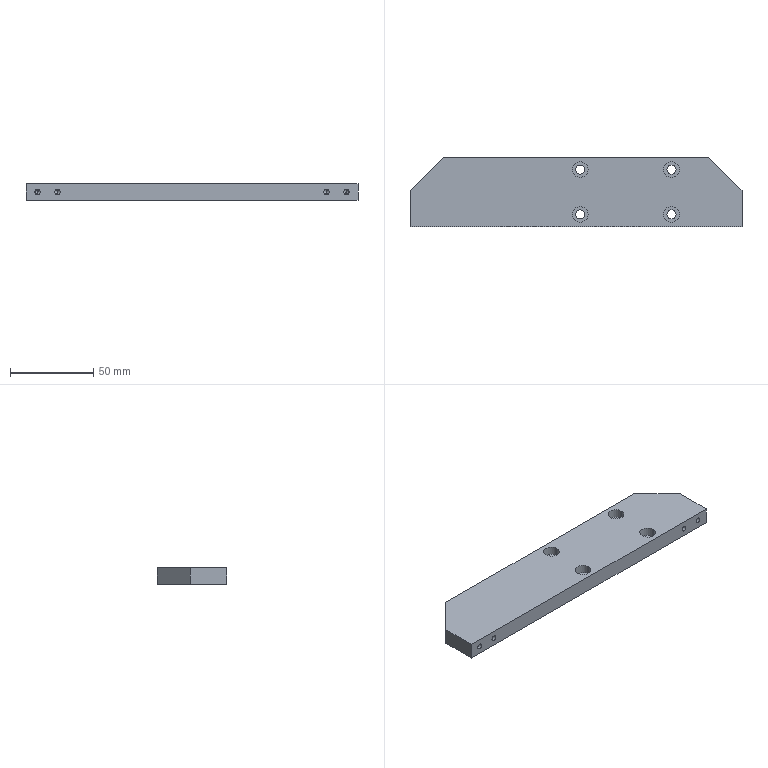Part | STEP file | CA-10-016Pusher Connecting Plate_Default | 1 solid | 44 faces | box 200 x 42 x 10 mm | volume 77675 mm3 | cylinder 24 | plane 12 | cone 8 | commonest cylinder face diameters 3.3 x8 5.5 x8 9.5 x8